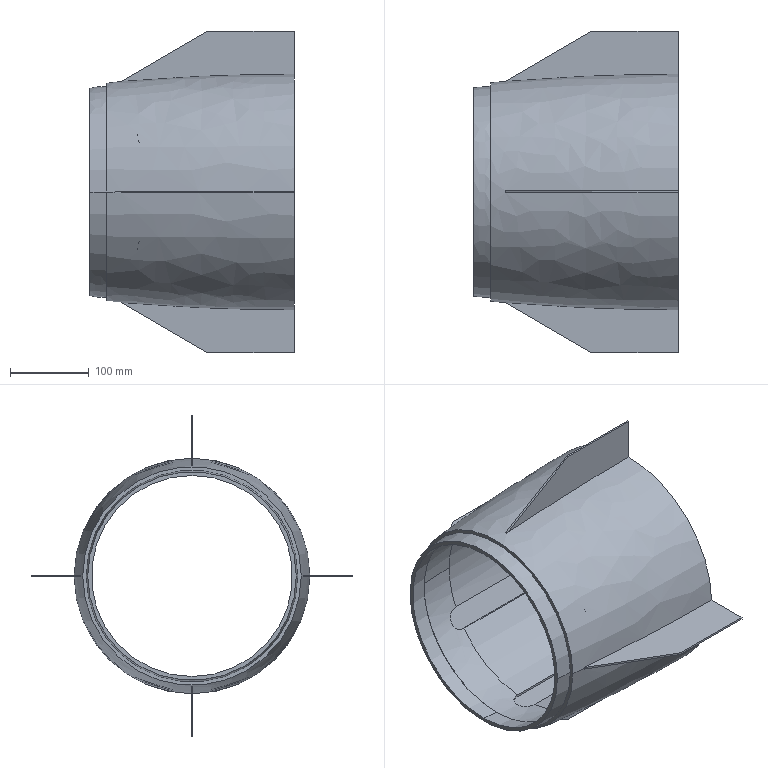Part | SolidWorks | features ICE 3, CirPattern 2, Revolution 2, RefAxis 1 | 1 solid | 68 faces | box 260.298 x 410 x 410 mm | volume 1987551 mm3 | plane 46 | cylinder 12 | spline 6 | cone 4 | commonest cylinder face diameters 30 x6 276.008 x6